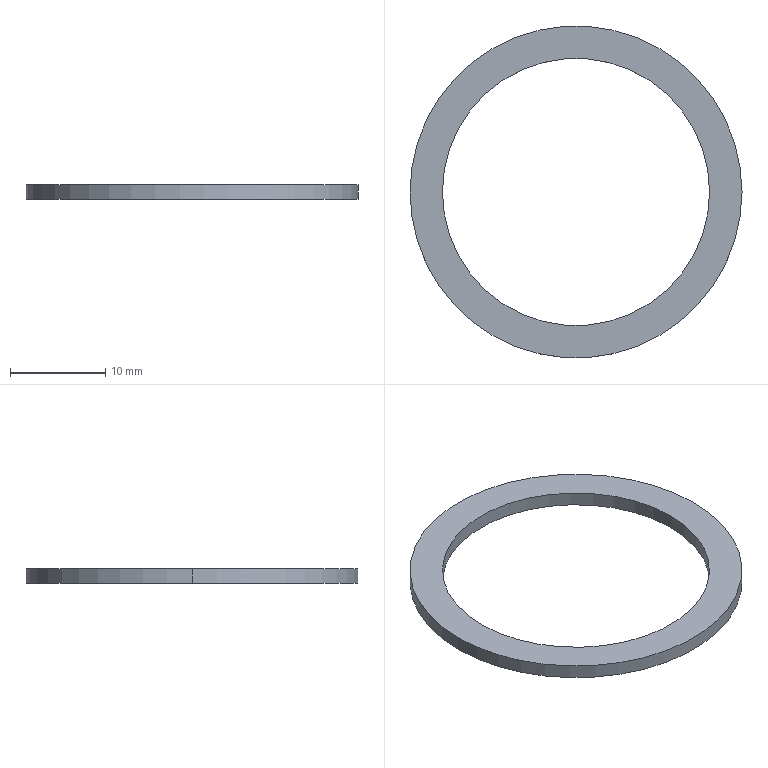Part | SolidWorks | features BaseBody 1 | 1 solid | 6 faces | box 34.8 x 34.8 x 1.5 mm | volume 503.095 mm3 | cylinder 4 | plane 2 | commonest cylinder face diameters 28 x2 34.8 x2
STEP:
#1=CARTESIAN_POINT('',(-17.4,0.,1.));
#2=VERTEX_POINT('',#1);
#3=CARTESIAN_POINT('',(17.4,0.,1.));
#4=VERTEX_POINT('',#3);
#5=CARTESIAN_POINT('',(0.,0.,1.));
#6=DIRECTION('',(0.,0.,-1.));
#7=DIRECTION('',(-1.,0.,0.));
#8=AXIS2_PLACEMENT_3D('',#5,#6,#7);
#9=CIRCLE('',#8,17.4);
#10=EDGE_CURVE('',#2,#4,#9,.T.);
#11=ORIENTED_EDGE('',*,*,#10,.T.);
#12=CARTESIAN_POINT('',(17.4,0.,-0.5));
#13=VERTEX_POINT('',#12);
#14=CARTESIAN_POINT('',(17.4,0.,1.));
#15=DIRECTION('',(0.,0.,-1.));
#16=VECTOR('',#15,1000.);
#17=LINE('',#14,#16);
#18=EDGE_CURVE('',#4,#13,#17,.T.);
#19=ORIENTED_EDGE('',*,*,#18,.T.);
#20=CARTESIAN_POINT('',(-17.4,0.,-0.5));
#21=VERTEX_POINT('',#20);
#22=CARTESIAN_POINT('',(0.,0.,-0.5));
#23=DIRECTION('',(0.,0.,1.));
#24=DIRECTION('',(-1.,0.,0.));
#25=AXIS2_PLACEMENT_3D('',#22,#23,#24);
#26=CIRCLE('',#25,17.4);
#27=EDGE_CURVE('',#13,#21,#26,.T.);
#28=ORIENTED_EDGE('',*,*,#27,.T.);
#29=CARTESIAN_POINT('',(-17.4,0.,1.));
#30=DIRECTION('',(0.,0.,-1.));
#31=VECTOR('',#30,1000.);
#32=LINE('',#29,#31);
#33=EDGE_CURVE('',#2,#21,#32,.T.);
#34=ORIENTED_EDGE('',*,*,#33,.F.);
#35=EDGE_LOOP('',(#11,#19,#28,#34));
#36=FACE_OUTER_BOUND('',#35,.T.);
#37=CARTESIAN_POINT('',(0.,0.,1.));
#38=DIRECTION('',(0.,0.,-1.));
#39=DIRECTION('',(-1.,0.,0.));
#40=AXIS2_PLACEMENT_3D('',#37,#38,#39);
#41=CYLINDRICAL_SURFACE('',#40,17.4);
#42=ADVANCED_FACE('',(#36),#41,.T.);
#43=CARTESIAN_POINT('',(14.,0.,-0.5));
#44=VERTEX_POINT('',#43);
#45=CARTESIAN_POINT('',(-14.,0.,-0.5));
#46=VERTEX_POINT('',#45);
#47=CARTESIAN_POINT('',(0.,0.,-0.5));
#48=DIRECTION('',(0.,0.,-1.));
#49=DIRECTION('',(1.,0.,0.));
#50=AXIS2_PLACEMENT_3D('',#47,#48,#49);
#51=CIRCLE('',#50,14.);
#52=EDGE_CURVE('',#44,#46,#51,.T.);
#53=ORIENTED_EDGE('',*,*,#52,.T.);
#54=CARTESIAN_POINT('',(-14.,0.,1.));
#55=VERTEX_POINT('',#54);
#56=CARTESIAN_POINT('',(-14.,0.,-9.));
#57=DIRECTION('',(0.,0.,1.));
#58=VECTOR('',#57,1000.);
#59=LINE('',#56,#58);
#60=EDGE_CURVE('',#46,#55,#59,.T.);
#61=ORIENTED_EDGE('',*,*,#60,.T.);
#62=CARTESIAN_POINT('',(14.,0.,1.));
#63=VERTEX_POINT('',#62);
#64=CARTESIAN_POINT('',(0.,0.,1.));
#65=DIRECTION('',(0.,0.,-1.));
#66=DIRECTION('',(1.,0.,0.));
#67=AXIS2_PLACEMENT_3D('',#64,#65,#66);
#68=CIRCLE('',#67,14.);
#69=EDGE_CURVE('',#63,#55,#68,.T.);
#70=ORIENTED_EDGE('',*,*,#69,.F.);
#71=CARTESIAN_POINT('',(14.,0.,-9.));
#72=DIRECTION('',(0.,0.,1.));
#73=VECTOR('',#72,1000.);
#74=LINE('',#71,#73);
#75=EDGE_CURVE('',#44,#63,#74,.T.);
#76=ORIENTED_EDGE('',*,*,#75,.F.);
#77=EDGE_LOOP('',(#53,#61,#70,#76));
#78=FACE_OUTER_BOUND('',#77,.T.);
#79=CARTESIAN_POINT('',(0.,0.,-9.));
#80=DIRECTION('',(0.,0.,1.));
#81=DIRECTION('',(1.,0.,0.));
#82=AXIS2_PLACEMENT_3D('',#79,#80,#81);
#83=CYLINDRICAL_SURFACE('',#82,14.);
#84=ADVANCED_FACE('',(#78),#83,.F.);
#85=CARTESIAN_POINT('',(0.,0.,-0.5));
#86=DIRECTION('',(0.,0.,1.));
#87=DIRECTION('',(-1.,0.,0.));
#88=AXIS2_PLACEMENT_3D('',#85,#86,#87);
#89=CIRCLE('',#88,17.4);
#90=EDGE_CURVE('',#21,#13,#89,.T.);
#91=ORIENTED_EDGE('',*,*,#90,.F.);
#92=ORIENTED_EDGE('',*,*,#27,.F.);
#93=EDGE_LOOP('',(#91,#92));
#94=FACE_OUTER_BOUND('',#93,.T.);
#95=ORIENTED_EDGE('',*,*,#52,.F.);
#96=CARTESIAN_POINT('',(0.,0.,-0.5));
#97=DIRECTION('',(0.,0.,-1.));
#98=DIRECTION('',(1.,0.,0.));
#99=AXIS2_PLACEMENT_3D('',#96,#97,#98);
#100=CIRCLE('',#99,14.);
#101=EDGE_CURVE('',#46,#44,#100,.T.);
#102=ORIENTED_EDGE('',*,*,#101,.F.);
#103=EDGE_LOOP('',(#95,#102));
#104=FACE_BOUND('',#103,.T.);
#105=CARTESIAN_POINT('',(0.,0.,-0.5));
#106=DIRECTION('',(0.,0.,1.));
#107=DIRECTION('',(1.,0.,0.));
#108=AXIS2_PLACEMENT_3D('',#105,#106,#107);
#109=PLANE('',#108);
#110=ADVANCED_FACE('',(#94,#104),#109,.F.);
#111=ORIENTED_EDGE('',*,*,#18,.F.);
#112=CARTESIAN_POINT('',(0.,0.,1.));
#113=DIRECTION('',(0.,0.,-1.));
#114=DIRECTION('',(-1.,0.,0.));
#115=AXIS2_PLACEMENT_3D('',#112,#113,#114);
#116=CIRCLE('',#115,17.4);
#117=EDGE_CURVE('',#4,#2,#116,.T.);
#118=ORIENTED_EDGE('',*,*,#117,.T.);
#119=ORIENTED_EDGE('',*,*,#33,.T.);
#120=ORIENTED_EDGE('',*,*,#90,.T.);
#121=EDGE_LOOP('',(#111,#118,#119,#120));
#122=FACE_OUTER_BOUND('',#121,.T.);
#123=CARTESIAN_POINT('',(0.,0.,1.));
#124=DIRECTION('',(0.,0.,-1.));
#125=DIRECTION('',(-1.,0.,0.));
#126=AXIS2_PLACEMENT_3D('',#123,#124,#125);
#127=CYLINDRICAL_SURFACE('',#126,17.4);
#128=ADVANCED_FACE('',(#122),#127,.T.);
#129=ORIENTED_EDGE('',*,*,#60,.F.);
#130=ORIENTED_EDGE('',*,*,#101,.T.);
#131=ORIENTED_EDGE('',*,*,#75,.T.);
#132=CARTESIAN_POINT('',(0.,0.,1.));
#133=DIRECTION('',(0.,0.,-1.));
#134=DIRECTION('',(1.,0.,0.));
#135=AXIS2_PLACEMENT_3D('',#132,#133,#134);
#136=CIRCLE('',#135,14.);
#137=EDGE_CURVE('',#55,#63,#136,.T.);
#138=ORIENTED_EDGE('',*,*,#137,.F.);
#139=EDGE_LOOP('',(#129,#130,#131,#138));
#140=FACE_OUTER_BOUND('',#139,.T.);
#141=CARTESIAN_POINT('',(0.,0.,-9.));
#142=DIRECTION('',(0.,0.,1.));
#143=DIRECTION('',(1.,0.,0.));
#144=AXIS2_PLACEMENT_3D('',#141,#142,#143);
#145=CYLINDRICAL_SURFACE('',#144,14.);
#146=ADVANCED_FACE('',(#140),#145,.F.);
#147=ORIENTED_EDGE('',*,*,#10,.F.);
#148=ORIENTED_EDGE('',*,*,#117,.F.);
#149=EDGE_LOOP('',(#147,#148));
#150=FACE_OUTER_BOUND('',#149,.T.);
#151=ORIENTED_EDGE('',*,*,#69,.T.);
#152=ORIENTED_EDGE('',*,*,#137,.T.);
#153=EDGE_LOOP('',(#151,#152));
#154=FACE_BOUND('',#153,.T.);
#155=CARTESIAN_POINT('',(0.,0.,1.));
#156=DIRECTION('',(0.,0.,1.));
#157=DIRECTION('',(1.,0.,0.));
#158=AXIS2_PLACEMENT_3D('',#155,#156,#157);
#159=PLANE('',#158);
#160=ADVANCED_FACE('',(#150,#154),#159,.T.);
#161=CLOSED_SHELL('',(#42,#84,#110,#128,#146,#160));
#162=MANIFOLD_SOLID_BREP('',#161);
#163=CARTESIAN_POINT('',(0.,0.,0.));
#164=DIRECTION('',(0.,0.,1.));
#165=DIRECTION('',(1.,0.,0.));
#166=AXIS2_PLACEMENT_3D('',#163,#164,#165);
#167=(LENGTH_UNIT()NAMED_UNIT(*)SI_UNIT(.MILLI.,.METRE.));
#168=UNCERTAINTY_MEASURE_WITH_UNIT(LENGTH_MEASURE(0.00001),#167,'','');
#169=(NAMED_UNIT(*)PLANE_ANGLE_UNIT()SI_UNIT($,.RADIAN.));
#170=(NAMED_UNIT(*)SI_UNIT($,.STERADIAN.)SOLID_ANGLE_UNIT());
#171=(GEOMETRIC_REPRESENTATION_CONTEXT(3)GLOBAL_UNCERTAINTY_ASSIGNED_CONTEXT((#168))GLOBAL_UNIT_ASSIGNED_CONTEXT((#167,#169,#170))REPRESENTATION_CONTEXT('',''));
#172=ADVANCED_BREP_SHAPE_REPRESENTATION('',(#162,#166),#171);